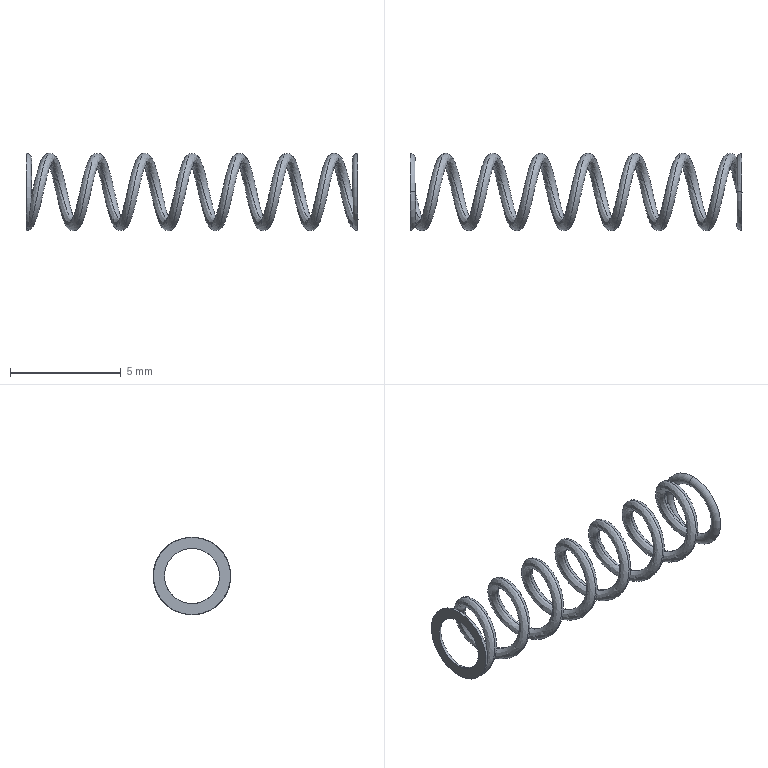Part | NX | features BREP 1 | 1 solid | 8 faces | box 15 x 3.5 x 3.5 mm | volume 14.439 mm3 | torus 4 | spline 2 | plane 2